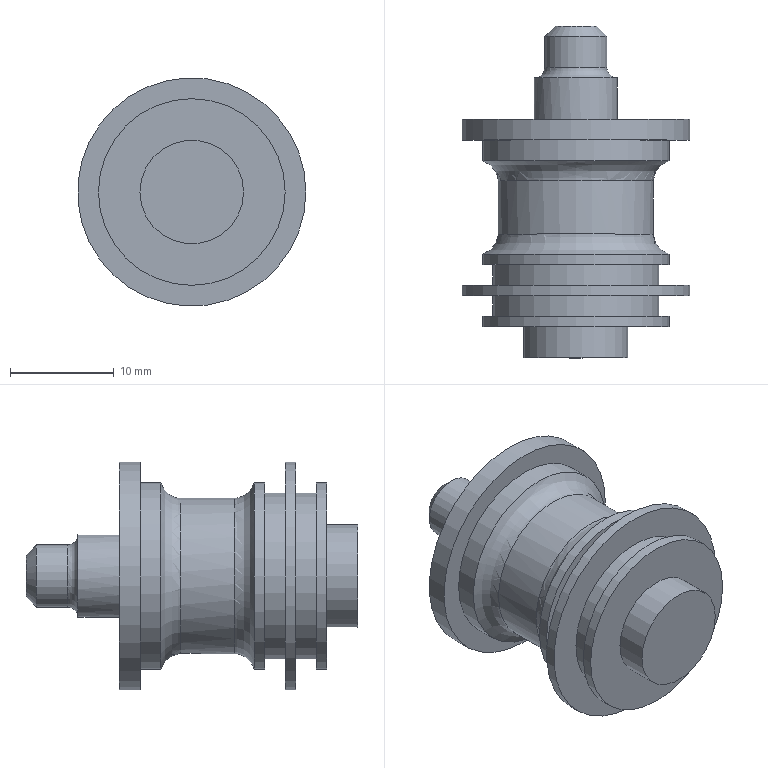Part | NX | features EXTRUDE 11, DATUM_CSYS 8, SKETCH 7, BLEND 3, CHAMFER 1 | 1 solid | 24 faces | box 22 x 32 x 22 mm | volume 5202 mm3 | cylinder 11 | plane 9 | torus 3 | cone 1 | commonest cylinder face diameters 18 x3 16 x2 22 x2 6 x1 8 x1 10 x1
STEP:
#1=CARTESIAN_POINT('',(4.,23.,0.));
#2=VERTEX_POINT('',#1);
#3=CARTESIAN_POINT('',(0.,23.,0.));
#4=DIRECTION('',(0.,-1.,0.));
#5=DIRECTION('',(1.,0.,0.));
#6=AXIS2_PLACEMENT_3D('',#3,#4,#5);
#7=CIRCLE('',#6,4.);
#8=EDGE_CURVE('',#2,#2,#7,.T.);
#9=ORIENTED_EDGE('',*,*,#8,.F.);
#10=EDGE_LOOP('',(#9));
#11=FACE_BOUND('',#10,.T.);
#12=CARTESIAN_POINT('',(4.,27.,0.));
#13=VERTEX_POINT('',#12);
#14=CARTESIAN_POINT('',(0.,27.,0.));
#15=DIRECTION('',(0.,-1.,0.));
#16=DIRECTION('',(1.,0.,0.));
#17=AXIS2_PLACEMENT_3D('',#14,#15,#16);
#18=CIRCLE('',#17,4.);
#19=EDGE_CURVE('',#13,#13,#18,.T.);
#20=ORIENTED_EDGE('',*,*,#19,.T.);
#21=EDGE_LOOP('',(#20));
#22=FACE_BOUND('',#21,.T.);
#23=CARTESIAN_POINT('',(0.,32.,0.));
#24=DIRECTION('',(0.,-1.,0.));
#25=DIRECTION('',(0.,0.,-1.));
#26=AXIS2_PLACEMENT_3D('',#23,#24,#25);
#27=CYLINDRICAL_SURFACE('',#26,4.);
#28=ADVANCED_FACE('',(#11,#22),#27,.T.);
#29=CARTESIAN_POINT('',(9.,10.,0.));
#30=VERTEX_POINT('',#29);
#31=CARTESIAN_POINT('',(0.,10.,0.));
#32=DIRECTION('',(0.,1.,0.));
#33=DIRECTION('',(1.,0.,0.));
#34=AXIS2_PLACEMENT_3D('',#31,#32,#33);
#35=CIRCLE('',#34,9.);
#36=EDGE_CURVE('',#30,#30,#35,.T.);
#37=ORIENTED_EDGE('',*,*,#36,.F.);
#38=EDGE_LOOP('',(#37));
#39=FACE_BOUND('',#38,.T.);
#40=CARTESIAN_POINT('',(9.,9.,0.));
#41=VERTEX_POINT('',#40);
#42=CARTESIAN_POINT('',(0.,9.,0.));
#43=DIRECTION('',(0.,1.,0.));
#44=DIRECTION('',(1.,0.,0.));
#45=AXIS2_PLACEMENT_3D('',#42,#43,#44);
#46=CIRCLE('',#45,9.);
#47=EDGE_CURVE('',#41,#41,#46,.T.);
#48=ORIENTED_EDGE('',*,*,#47,.T.);
#49=EDGE_LOOP('',(#48));
#50=FACE_BOUND('',#49,.T.);
#51=CARTESIAN_POINT('',(0.,5.,0.));
#52=DIRECTION('',(0.,1.,0.));
#53=DIRECTION('',(0.,0.,1.));
#54=AXIS2_PLACEMENT_3D('',#51,#52,#53);
#55=CYLINDRICAL_SURFACE('',#54,9.);
#56=ADVANCED_FACE('',(#39,#50),#55,.T.);
#57=CARTESIAN_POINT('',(0.,11.936,-7.5));
#58=VERTEX_POINT('',#57);
#59=CARTESIAN_POINT('',(0.,11.936,0.));
#60=DIRECTION('',(0.,-1.,0.));
#61=DIRECTION('',(0.,0.,-1.));
#62=AXIS2_PLACEMENT_3D('',#59,#60,#61);
#63=CIRCLE('',#62,7.5);
#64=EDGE_CURVE('',#58,#58,#63,.F.);
#65=ORIENTED_EDGE('',*,*,#64,.T.);
#66=EDGE_LOOP('',(#65));
#67=FACE_BOUND('',#66,.T.);
#68=CARTESIAN_POINT('',(0.,17.064,7.5));
#69=VERTEX_POINT('',#68);
#70=CARTESIAN_POINT('',(0.,17.064,0.));
#71=DIRECTION('',(0.,1.,0.));
#72=DIRECTION('',(0.,0.,1.));
#73=AXIS2_PLACEMENT_3D('',#70,#71,#72);
#74=CIRCLE('',#73,7.5);
#75=EDGE_CURVE('',#69,#69,#74,.F.);
#76=ORIENTED_EDGE('',*,*,#75,.T.);
#77=EDGE_LOOP('',(#76));
#78=FACE_BOUND('',#77,.T.);
#79=CARTESIAN_POINT('',(0.,10.,0.));
#80=DIRECTION('',(0.,1.,0.));
#81=DIRECTION('',(0.,0.,1.));
#82=AXIS2_PLACEMENT_3D('',#79,#80,#81);
#83=CYLINDRICAL_SURFACE('',#82,7.5);
#84=ADVANCED_FACE('',(#67,#78),#83,.T.);
#85=ORIENTED_EDGE('',*,*,#8,.T.);
#86=EDGE_LOOP('',(#85));
#87=FACE_BOUND('',#86,.T.);
#88=CARTESIAN_POINT('',(11.,23.,0.));
#89=VERTEX_POINT('',#88);
#90=CARTESIAN_POINT('',(0.,23.,0.));
#91=DIRECTION('',(0.,-1.,0.));
#92=DIRECTION('',(1.,0.,0.));
#93=AXIS2_PLACEMENT_3D('',#90,#91,#92);
#94=CIRCLE('',#93,11.);
#95=EDGE_CURVE('',#89,#89,#94,.T.);
#96=ORIENTED_EDGE('',*,*,#95,.F.);
#97=EDGE_LOOP('',(#96));
#98=FACE_BOUND('',#97,.T.);
#99=CARTESIAN_POINT('',(0.,23.,0.));
#100=DIRECTION('',(0.,-1.,0.));
#101=DIRECTION('',(0.,0.,-1.));
#102=AXIS2_PLACEMENT_3D('',#99,#100,#101);
#103=PLANE('',#102);
#104=ADVANCED_FACE('',(#87,#98),#103,.F.);
#105=CARTESIAN_POINT('',(11.,21.,0.));
#106=VERTEX_POINT('',#105);
#107=CARTESIAN_POINT('',(0.,21.,0.));
#108=DIRECTION('',(0.,-1.,0.));
#109=DIRECTION('',(1.,0.,0.));
#110=AXIS2_PLACEMENT_3D('',#107,#108,#109);
#111=CIRCLE('',#110,11.);
#112=EDGE_CURVE('',#106,#106,#111,.T.);
#113=ORIENTED_EDGE('',*,*,#112,.F.);
#114=EDGE_LOOP('',(#113));
#115=FACE_BOUND('',#114,.T.);
#116=ORIENTED_EDGE('',*,*,#95,.T.);
#117=EDGE_LOOP('',(#116));
#118=FACE_BOUND('',#117,.T.);
#119=CARTESIAN_POINT('',(0.,23.,0.));
#120=DIRECTION('',(0.,-1.,0.));
#121=DIRECTION('',(0.,0.,-1.));
#122=AXIS2_PLACEMENT_3D('',#119,#120,#121);
#123=CYLINDRICAL_SURFACE('',#122,11.);
#124=ADVANCED_FACE('',(#115,#118),#123,.T.);
#125=ORIENTED_EDGE('',*,*,#112,.T.);
#126=EDGE_LOOP('',(#125));
#127=FACE_BOUND('',#126,.T.);
#128=CARTESIAN_POINT('',(9.,21.,0.));
#129=VERTEX_POINT('',#128);
#130=CARTESIAN_POINT('',(0.,21.,0.));
#131=DIRECTION('',(0.,1.,0.));
#132=DIRECTION('',(1.,0.,0.));
#133=AXIS2_PLACEMENT_3D('',#130,#131,#132);
#134=CIRCLE('',#133,9.);
#135=EDGE_CURVE('',#129,#129,#134,.F.);
#136=ORIENTED_EDGE('',*,*,#135,.F.);
#137=EDGE_LOOP('',(#136));
#138=FACE_BOUND('',#137,.T.);
#139=CARTESIAN_POINT('',(0.,21.,0.));
#140=DIRECTION('',(0.,-1.,0.));
#141=DIRECTION('',(0.,0.,-1.));
#142=AXIS2_PLACEMENT_3D('',#139,#140,#141);
#143=PLANE('',#142);
#144=ADVANCED_FACE('',(#127,#138),#143,.T.);
#145=ORIENTED_EDGE('',*,*,#135,.T.);
#146=EDGE_LOOP('',(#145));
#147=FACE_BOUND('',#146,.T.);
#148=CARTESIAN_POINT('',(9.,19.,0.));
#149=VERTEX_POINT('',#148);
#150=CARTESIAN_POINT('',(0.,19.,0.));
#151=DIRECTION('',(0.,1.,0.));
#152=DIRECTION('',(1.,0.,0.));
#153=AXIS2_PLACEMENT_3D('',#150,#151,#152);
#154=CIRCLE('',#153,9.);
#155=EDGE_CURVE('',#149,#149,#154,.T.);
#156=ORIENTED_EDGE('',*,*,#155,.T.);
#157=EDGE_LOOP('',(#156));
#158=FACE_BOUND('',#157,.T.);
#159=CARTESIAN_POINT('',(0.,5.,0.));
#160=DIRECTION('',(0.,1.,0.));
#161=DIRECTION('',(0.,0.,1.));
#162=AXIS2_PLACEMENT_3D('',#159,#160,#161);
#163=CYLINDRICAL_SURFACE('',#162,9.);
#164=ADVANCED_FACE('',(#147,#158),#163,.T.);
#165=CARTESIAN_POINT('',(8.,7.,0.));
#166=VERTEX_POINT('',#165);
#167=CARTESIAN_POINT('',(0.,7.,0.));
#168=DIRECTION('',(0.,1.,0.));
#169=DIRECTION('',(1.,0.,0.));
#170=AXIS2_PLACEMENT_3D('',#167,#168,#169);
#171=CIRCLE('',#170,8.);
#172=EDGE_CURVE('',#166,#166,#171,.T.);
#173=ORIENTED_EDGE('',*,*,#172,.T.);
#174=EDGE_LOOP('',(#173));
#175=FACE_BOUND('',#174,.T.);
#176=CARTESIAN_POINT('',(8.,9.,0.));
#177=VERTEX_POINT('',#176);
#178=CARTESIAN_POINT('',(0.,9.,0.));
#179=DIRECTION('',(0.,1.,0.));
#180=DIRECTION('',(1.,0.,0.));
#181=AXIS2_PLACEMENT_3D('',#178,#179,#180);
#182=CIRCLE('',#181,8.);
#183=EDGE_CURVE('',#177,#177,#182,.T.);
#184=ORIENTED_EDGE('',*,*,#183,.F.);
#185=EDGE_LOOP('',(#184));
#186=FACE_BOUND('',#185,.T.);
#187=CARTESIAN_POINT('',(0.,7.,0.));
#188=DIRECTION('',(0.,1.,0.));
#189=DIRECTION('',(0.,0.,1.));
#190=AXIS2_PLACEMENT_3D('',#187,#188,#189);
#191=CYLINDRICAL_SURFACE('',#190,8.);
#192=ADVANCED_FACE('',(#175,#186),#191,.T.);
#193=ORIENTED_EDGE('',*,*,#172,.F.);
#194=EDGE_LOOP('',(#193));
#195=FACE_BOUND('',#194,.T.);
#196=CARTESIAN_POINT('',(11.,7.,0.));
#197=VERTEX_POINT('',#196);
#198=CARTESIAN_POINT('',(0.,7.,0.));
#199=DIRECTION('',(0.,-1.,0.));
#200=DIRECTION('',(1.,0.,0.));
#201=AXIS2_PLACEMENT_3D('',#198,#199,#200);
#202=CIRCLE('',#201,11.);
#203=EDGE_CURVE('',#197,#197,#202,.T.);
#204=ORIENTED_EDGE('',*,*,#203,.F.);
#205=EDGE_LOOP('',(#204));
#206=FACE_BOUND('',#205,.T.);
#207=CARTESIAN_POINT('',(0.,7.,0.));
#208=DIRECTION('',(0.,1.,0.));
#209=DIRECTION('',(0.,0.,1.));
#210=AXIS2_PLACEMENT_3D('',#207,#208,#209);
#211=PLANE('',#210);
#212=ADVANCED_FACE('',(#195,#206),#211,.T.);
#213=ORIENTED_EDGE('',*,*,#47,.F.);
#214=EDGE_LOOP('',(#213));
#215=FACE_BOUND('',#214,.T.);
#216=ORIENTED_EDGE('',*,*,#183,.T.);
#217=EDGE_LOOP('',(#216));
#218=FACE_BOUND('',#217,.T.);
#219=CARTESIAN_POINT('',(0.,9.,0.));
#220=DIRECTION('',(0.,1.,0.));
#221=DIRECTION('',(0.,0.,1.));
#222=AXIS2_PLACEMENT_3D('',#219,#220,#221);
#223=PLANE('',#222);
#224=ADVANCED_FACE('',(#215,#218),#223,.F.);
#225=CARTESIAN_POINT('',(11.,6.,0.));
#226=VERTEX_POINT('',#225);
#227=CARTESIAN_POINT('',(0.,6.,0.));
#228=DIRECTION('',(0.,-1.,0.));
#229=DIRECTION('',(1.,0.,0.));
#230=AXIS2_PLACEMENT_3D('',#227,#228,#229);
#231=CIRCLE('',#230,11.);
#232=EDGE_CURVE('',#226,#226,#231,.T.);
#233=ORIENTED_EDGE('',*,*,#232,.F.);
#234=EDGE_LOOP('',(#233));
#235=FACE_BOUND('',#234,.T.);
#236=ORIENTED_EDGE('',*,*,#203,.T.);
#237=EDGE_LOOP('',(#236));
#238=FACE_BOUND('',#237,.T.);
#239=CARTESIAN_POINT('',(0.,6.,0.));
#240=DIRECTION('',(0.,1.,0.));
#241=DIRECTION('',(0.,0.,1.));
#242=AXIS2_PLACEMENT_3D('',#239,#240,#241);
#243=CYLINDRICAL_SURFACE('',#242,11.);
#244=ADVANCED_FACE('',(#235,#238),#243,.T.);
#245=CARTESIAN_POINT('',(9.,3.,0.));
#246=VERTEX_POINT('',#245);
#247=CARTESIAN_POINT('',(0.,3.,0.));
#248=DIRECTION('',(0.,1.,0.));
#249=DIRECTION('',(1.,0.,0.));
#250=AXIS2_PLACEMENT_3D('',#247,#248,#249);
#251=CIRCLE('',#250,9.);
#252=EDGE_CURVE('',#246,#246,#251,.T.);
#253=ORIENTED_EDGE('',*,*,#252,.F.);
#254=EDGE_LOOP('',(#253));
#255=FACE_BOUND('',#254,.T.);
#256=CARTESIAN_POINT('',(5.,3.,0.));
#257=VERTEX_POINT('',#256);
#258=CARTESIAN_POINT('',(0.,3.,0.));
#259=DIRECTION('',(0.,1.,0.));
#260=DIRECTION('',(1.,0.,0.));
#261=AXIS2_PLACEMENT_3D('',#258,#259,#260);
#262=CIRCLE('',#261,5.);
#263=EDGE_CURVE('',#257,#257,#262,.T.);
#264=ORIENTED_EDGE('',*,*,#263,.T.);
#265=EDGE_LOOP('',(#264));
#266=FACE_BOUND('',#265,.T.);
#267=CARTESIAN_POINT('',(0.,3.,0.));
#268=DIRECTION('',(0.,1.,0.));
#269=DIRECTION('',(0.,0.,1.));
#270=AXIS2_PLACEMENT_3D('',#267,#268,#269);
#271=PLANE('',#270);
#272=ADVANCED_FACE('',(#255,#266),#271,.F.);
#273=ORIENTED_EDGE('',*,*,#252,.T.);
#274=EDGE_LOOP('',(#273));
#275=FACE_BOUND('',#274,.T.);
#276=CARTESIAN_POINT('',(9.,4.,0.));
#277=VERTEX_POINT('',#276);
#278=CARTESIAN_POINT('',(0.,4.,0.));
#279=DIRECTION('',(0.,1.,0.));
#280=DIRECTION('',(1.,0.,0.));
#281=AXIS2_PLACEMENT_3D('',#278,#279,#280);
#282=CIRCLE('',#281,9.);
#283=EDGE_CURVE('',#277,#277,#282,.T.);
#284=ORIENTED_EDGE('',*,*,#283,.F.);
#285=EDGE_LOOP('',(#284));
#286=FACE_BOUND('',#285,.T.);
#287=CARTESIAN_POINT('',(0.,3.,0.));
#288=DIRECTION('',(0.,1.,0.));
#289=DIRECTION('',(0.,0.,1.));
#290=AXIS2_PLACEMENT_3D('',#287,#288,#289);
#291=CYLINDRICAL_SURFACE('',#290,9.);
#292=ADVANCED_FACE('',(#275,#286),#291,.T.);
#293=ORIENTED_EDGE('',*,*,#283,.T.);
#294=EDGE_LOOP('',(#293));
#295=FACE_BOUND('',#294,.T.);
#296=CARTESIAN_POINT('',(8.,4.,0.));
#297=VERTEX_POINT('',#296);
#298=CARTESIAN_POINT('',(0.,4.,0.));
#299=DIRECTION('',(0.,-1.,0.));
#300=DIRECTION('',(1.,0.,0.));
#301=AXIS2_PLACEMENT_3D('',#298,#299,#300);
#302=CIRCLE('',#301,8.);
#303=EDGE_CURVE('',#297,#297,#302,.F.);
#304=ORIENTED_EDGE('',*,*,#303,.F.);
#305=EDGE_LOOP('',(#304));
#306=FACE_BOUND('',#305,.T.);
#307=CARTESIAN_POINT('',(0.,4.,0.));
#308=DIRECTION('',(0.,-1.,0.));
#309=DIRECTION('',(0.,0.,-1.));
#310=AXIS2_PLACEMENT_3D('',#307,#308,#309);
#311=PLANE('',#310);
#312=ADVANCED_FACE('',(#295,#306),#311,.F.);
#313=ORIENTED_EDGE('',*,*,#303,.T.);
#314=EDGE_LOOP('',(#313));
#315=FACE_BOUND('',#314,.T.);
#316=CARTESIAN_POINT('',(8.,6.,0.));
#317=VERTEX_POINT('',#316);
#318=CARTESIAN_POINT('',(0.,6.,0.));
#319=DIRECTION('',(0.,-1.,0.));
#320=DIRECTION('',(1.,0.,0.));
#321=AXIS2_PLACEMENT_3D('',#318,#319,#320);
#322=CIRCLE('',#321,8.);
#323=EDGE_CURVE('',#317,#317,#322,.F.);
#324=ORIENTED_EDGE('',*,*,#323,.F.);
#325=EDGE_LOOP('',(#324));
#326=FACE_BOUND('',#325,.T.);
#327=CARTESIAN_POINT('',(0.,4.,0.));
#328=DIRECTION('',(0.,1.,0.));
#329=DIRECTION('',(0.,0.,1.));
#330=AXIS2_PLACEMENT_3D('',#327,#328,#329);
#331=CYLINDRICAL_SURFACE('',#330,8.);
#332=ADVANCED_FACE('',(#315,#326),#331,.T.);
#333=ORIENTED_EDGE('',*,*,#323,.T.);
#334=EDGE_LOOP('',(#333));
#335=FACE_BOUND('',#334,.T.);
#336=ORIENTED_EDGE('',*,*,#232,.T.);
#337=EDGE_LOOP('',(#336));
#338=FACE_BOUND('',#337,.T.);
#339=CARTESIAN_POINT('',(0.,6.,0.));
#340=DIRECTION('',(0.,-1.,0.));
#341=DIRECTION('',(0.,0.,-1.));
#342=AXIS2_PLACEMENT_3D('',#339,#340,#341);
#343=PLANE('',#342);
#344=ADVANCED_FACE('',(#335,#338),#343,.T.);
#345=ORIENTED_EDGE('',*,*,#155,.F.);
#346=EDGE_LOOP('',(#345));
#347=FACE_BOUND('',#346,.T.);
#348=ORIENTED_EDGE('',*,*,#75,.F.);
#349=EDGE_LOOP('',(#348));
#350=FACE_BOUND('',#349,.T.);
#351=CARTESIAN_POINT('',(0.,17.064,0.));
#352=DIRECTION('',(0.,1.,0.));
#353=DIRECTION('',(0.,0.,1.));
#354=AXIS2_PLACEMENT_3D('',#351,#352,#353);
#355=TOROIDAL_SURFACE('',#354,9.5,2.);
#356=ADVANCED_FACE('',(#347,#350),#355,.F.);
#357=ORIENTED_EDGE('',*,*,#64,.F.);
#358=EDGE_LOOP('',(#357));
#359=FACE_BOUND('',#358,.T.);
#360=ORIENTED_EDGE('',*,*,#36,.T.);
#361=EDGE_LOOP('',(#360));
#362=FACE_BOUND('',#361,.T.);
#363=CARTESIAN_POINT('',(0.,11.936,0.));
#364=DIRECTION('',(0.,-1.,0.));
#365=DIRECTION('',(0.,0.,-1.));
#366=AXIS2_PLACEMENT_3D('',#363,#364,#365);
#367=TOROIDAL_SURFACE('',#366,9.5,2.);
#368=ADVANCED_FACE('',(#359,#362),#367,.F.);
#369=CARTESIAN_POINT('',(0.,31.,-3.));
#370=VERTEX_POINT('',#369);
#371=CARTESIAN_POINT('',(0.,31.,0.));
#372=DIRECTION('',(0.,-1.,0.));
#373=DIRECTION('',(0.,0.,-1.));
#374=AXIS2_PLACEMENT_3D('',#371,#372,#373);
#375=CIRCLE('',#374,3.);
#376=EDGE_CURVE('',#370,#370,#375,.T.);
#377=ORIENTED_EDGE('',*,*,#376,.T.);
#378=EDGE_LOOP('',(#377));
#379=FACE_BOUND('',#378,.T.);
#380=CARTESIAN_POINT('',(0.,28.,-3.));
#381=VERTEX_POINT('',#380);
#382=CARTESIAN_POINT('',(0.,28.,0.));
#383=DIRECTION('',(0.,-1.,0.));
#384=DIRECTION('',(0.,0.,-1.));
#385=AXIS2_PLACEMENT_3D('',#382,#383,#384);
#386=CIRCLE('',#385,3.);
#387=EDGE_CURVE('',#381,#381,#386,.F.);
#388=ORIENTED_EDGE('',*,*,#387,.T.);
#389=EDGE_LOOP('',(#388));
#390=FACE_BOUND('',#389,.T.);
#391=CARTESIAN_POINT('',(0.,27.,0.));
#392=DIRECTION('',(0.,1.,0.));
#393=DIRECTION('',(0.,0.,1.));
#394=AXIS2_PLACEMENT_3D('',#391,#392,#393);
#395=CYLINDRICAL_SURFACE('',#394,3.);
#396=ADVANCED_FACE('',(#379,#390),#395,.T.);
#397=CARTESIAN_POINT('',(0.,32.,-2.));
#398=VERTEX_POINT('',#397);
#399=CARTESIAN_POINT('',(0.,32.,0.));
#400=DIRECTION('',(0.,-1.,0.));
#401=DIRECTION('',(0.,0.,-1.));
#402=AXIS2_PLACEMENT_3D('',#399,#400,#401);
#403=CIRCLE('',#402,2.);
#404=EDGE_CURVE('',#398,#398,#403,.F.);
#405=ORIENTED_EDGE('',*,*,#404,.T.);
#406=EDGE_LOOP('',(#405));
#407=FACE_BOUND('',#406,.T.);
#408=CARTESIAN_POINT('',(0.,32.,0.));
#409=DIRECTION('',(0.,-1.,0.));
#410=DIRECTION('',(0.,0.,-1.));
#411=AXIS2_PLACEMENT_3D('',#408,#409,#410);
#412=PLANE('',#411);
#413=ADVANCED_FACE('',(#407),#412,.F.);
#414=ORIENTED_EDGE('',*,*,#19,.F.);
#415=EDGE_LOOP('',(#414));
#416=FACE_BOUND('',#415,.T.);
#417=ORIENTED_EDGE('',*,*,#387,.F.);
#418=EDGE_LOOP('',(#417));
#419=FACE_BOUND('',#418,.T.);
#420=CARTESIAN_POINT('',(0.,28.,0.));
#421=DIRECTION('',(0.,-1.,0.));
#422=DIRECTION('',(0.,0.,-1.));
#423=AXIS2_PLACEMENT_3D('',#420,#421,#422);
#424=TOROIDAL_SURFACE('',#423,4.,1.);
#425=ADVANCED_FACE('',(#416,#419),#424,.F.);
#426=ORIENTED_EDGE('',*,*,#404,.F.);
#427=EDGE_LOOP('',(#426));
#428=FACE_BOUND('',#427,.T.);
#429=ORIENTED_EDGE('',*,*,#376,.F.);
#430=EDGE_LOOP('',(#429));
#431=FACE_BOUND('',#430,.T.);
#432=CARTESIAN_POINT('',(0.,31.,0.));
#433=DIRECTION('',(0.,-1.,0.));
#434=DIRECTION('',(0.,0.,-1.));
#435=AXIS2_PLACEMENT_3D('',#432,#433,#434);
#436=CONICAL_SURFACE('',#435,3.,0.7854);
#437=ADVANCED_FACE('',(#428,#431),#436,.T.);
#438=ORIENTED_EDGE('',*,*,#263,.F.);
#439=EDGE_LOOP('',(#438));
#440=FACE_BOUND('',#439,.T.);
#441=CARTESIAN_POINT('',(5.,0.,0.));
#442=VERTEX_POINT('',#441);
#443=CARTESIAN_POINT('',(0.,0.,0.));
#444=DIRECTION('',(0.,1.,0.));
#445=DIRECTION('',(1.,0.,0.));
#446=AXIS2_PLACEMENT_3D('',#443,#444,#445);
#447=CIRCLE('',#446,5.);
#448=EDGE_CURVE('',#442,#442,#447,.T.);
#449=ORIENTED_EDGE('',*,*,#448,.T.);
#450=EDGE_LOOP('',(#449));
#451=FACE_BOUND('',#450,.T.);
#452=CARTESIAN_POINT('',(0.,3.,0.));
#453=DIRECTION('',(0.,-1.,0.));
#454=DIRECTION('',(0.,0.,-1.));
#455=AXIS2_PLACEMENT_3D('',#452,#453,#454);
#456=CYLINDRICAL_SURFACE('',#455,5.);
#457=ADVANCED_FACE('',(#440,#451),#456,.T.);
#458=ORIENTED_EDGE('',*,*,#448,.F.);
#459=EDGE_LOOP('',(#458));
#460=FACE_BOUND('',#459,.T.);
#461=CARTESIAN_POINT('',(0.,0.,0.));
#462=DIRECTION('',(0.,-1.,0.));
#463=DIRECTION('',(0.,0.,-1.));
#464=AXIS2_PLACEMENT_3D('',#461,#462,#463);
#465=PLANE('',#464);
#466=ADVANCED_FACE('',(#460),#465,.T.);
#467=CLOSED_SHELL('',(#28,#56,#84,#104,#124,#144,#164,#192,#212,#224,#244,#272,#292,#312,#332,#344,#356,#368,#396,#413,#425,#437,#457,#466));
#468=MANIFOLD_SOLID_BREP('',#467);
#469=(LENGTH_UNIT()NAMED_UNIT(*)SI_UNIT(.MILLI.,.METRE.));
#470=UNCERTAINTY_MEASURE_WITH_UNIT(LENGTH_MEASURE(0.00001),#469,'','');
#471=(NAMED_UNIT(*)PLANE_ANGLE_UNIT()SI_UNIT($,.RADIAN.));
#472=(NAMED_UNIT(*)SI_UNIT($,.STERADIAN.)SOLID_ANGLE_UNIT());
#473=(GEOMETRIC_REPRESENTATION_CONTEXT(3)GLOBAL_UNCERTAINTY_ASSIGNED_CONTEXT((#470))GLOBAL_UNIT_ASSIGNED_CONTEXT((#469,#471,#472))REPRESENTATION_CONTEXT('',''));
#474=ADVANCED_BREP_SHAPE_REPRESENTATION('',(#468),#473);